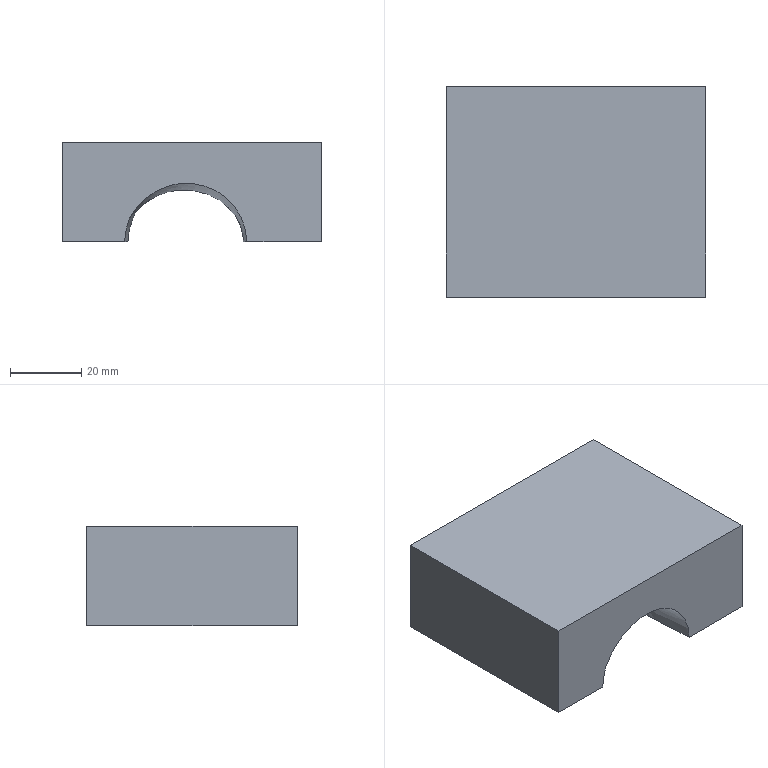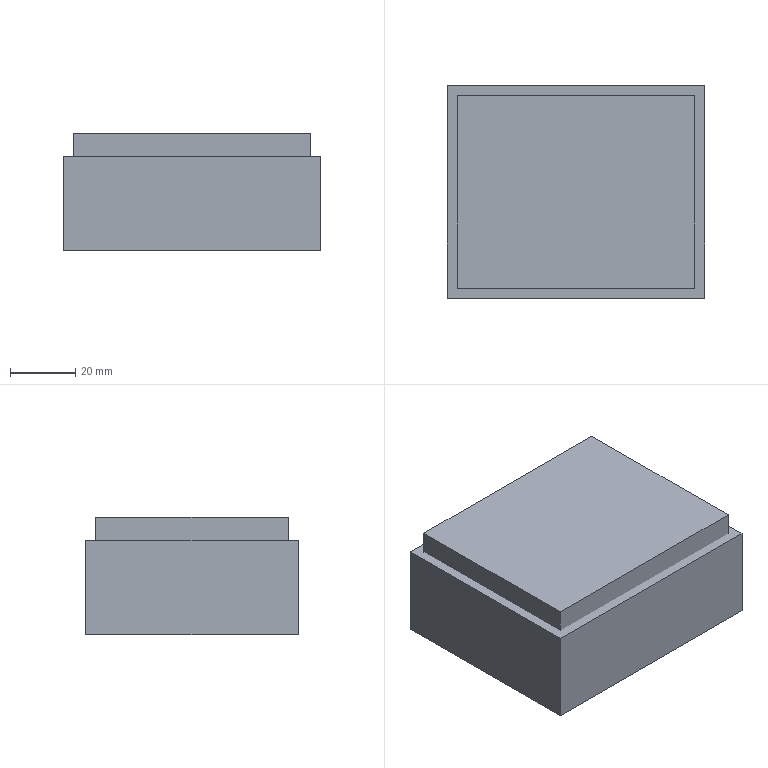CAM job | NX | 3-axis milling, drilling | part box 72.744 x 59.015 x 27.972 mm | stock box 78.744 x 65.015 x 35.972 mm
Tools:
number,name,description,diameter,corner_radius,flute_length,length,flutes
3,D63,Milling Tool-5 Parameters,63.0,0.0,50.0,75.0,2
4,D10,Milling Tool-5 Parameters,10.0,0.0,50.0,75.0,2
14,D10JING,Milling Tool-5 Parameters,10.0,0.0,50.0,75.0,2
1,D6A45,Milling Tool-5 Parameters,6.0,0.0,3.0,3.0,2
13,4.2ZT,Drilling Tool,4.2,0.0,35.0,50.0,2
12,6.0ZT,Drilling Tool,6.0,0.0,35.0,50.0,2
16,D6,Milling Tool-5 Parameters,6.0,0.0,50.0,75.0,2
11,R2,Milling Tool-5 Parameters,4.0,2.0,50.0,75.0,2
Operations:
program,operation,operation_type,tool,method,geometry_group,spindle_rpm,surface_speed,feed_per_tooth,feed_cut,feed_plunge,cut_length_mm,path_length_mm,cut_time_min,machine_time_min
1,FLOOR_WALL,VolumeBased25DMillingOperation,D63,METHOD,A,6500.0,1286.0,0.1154,1500.0,100.0,153.744,207.744,0.1025,0.1079
1,ADAPTIVE_MILLING,CavityMilling,D10,METHOD,A,9500.0,298.0,0.1579,3000.0,1000.0,1290.001,1511.439,0.434,0.4561
1,ZLEVEL_PROFILE_COPY_COPY,ZLevelMilling,D10JING,METHOD,A,9500.0,298.0,0.0632,1200.0,1000.0,596.127,712.251,0.4973,0.5089
1,ZLEVEL_PROFILE_1,ZLevelMilling,D6A45,METHOD,A,9500.0,179.0,0.0658,1250.0,100.0,275.863,334.863,0.2207,0.2266
2,FLOOR_WALL_COPY_1,VolumeBased25DMillingOperation,D63,METHOD,B,6500.0,1286.0,0.1154,1500.0,100.0,1181.948,2548.356,0.788,0.9246
2,FLOOR_WALL_COPY,VolumeBased25DMillingOperation,D63,METHOD,B,6500.0,1286.0,0.1154,1500.0,100.0,147.744,201.744,0.0985,0.1039
2,DRILLING,Operation,D6A45,METHOD,B,5000.0,94.0,0.025,250.0,0.0,16.0,184.769,0.064,0.0809
2,DRILLING_COPY_COPY,Operation,4.2ZT,METHOD,B,2000.0,37.0,0.0375,150.0,0.0,38.524,188.838,0.2568,0.2719
2,DRILLING_COPY_COPY_1,Operation,6.0ZT,METHOD,B,2000.0,37.0,0.0375,150.0,0.0,19.605,162.837,0.1307,0.145
2,ZLEVEL_PROFILE,ZLevelMilling,D10,METHOD,B,9500.0,298.0,0.1579,3000.0,1000.0,5412.909,5805.119,1.822,1.861
2,ZLEVEL_PROFILE_COPY,ZLevelMilling,D6,METHOD,B,9500.0,179.0,0.1316,2500.0,1000.0,924.403,1765.503,0.3979,0.482
2,FIXED_CONTOUR,SurfaceContour,R2,METHOD,B,9500.0,298.0,0.1579,3000.0,1000.0,50537.873,50591.772,16.856,16.861
2,ZLEVEL_PROFILE_1_COPY,ZLevelMilling,D6A45,METHOD,B,9500.0,179.0,0.0658,1250.0,100.0,399.158,940.561,0.3193,0.3735